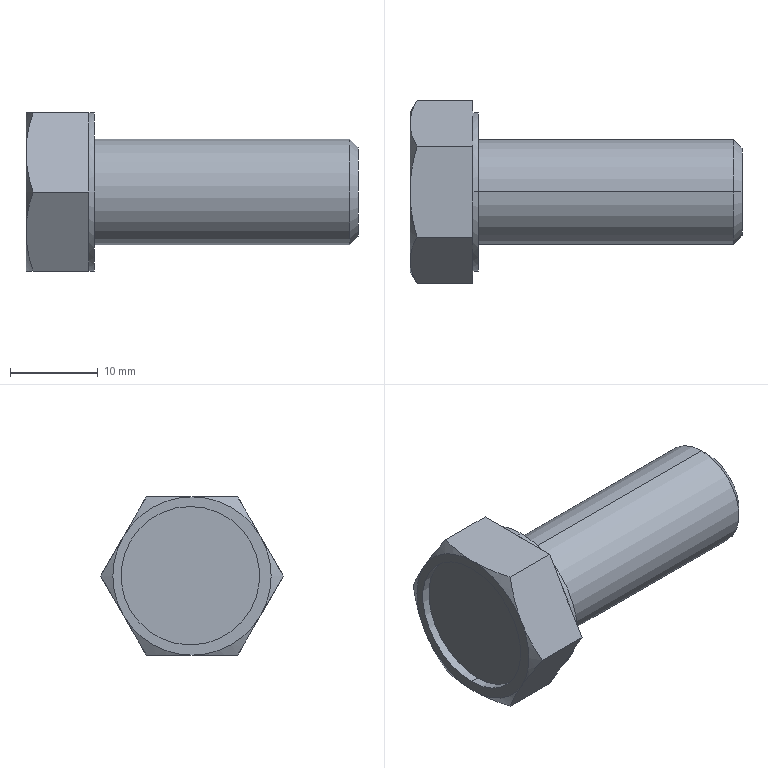Part | STEP file | formed hex screw_am_B18.2.3.2M - Formed hex screw, M12 x 1.75 x 30 --30WN | 1 solid | 30 faces | box 37.76 x 20.785 x 18 mm | volume 5343 mm3 | plane 16 | cone 8 | cylinder 6 | commonest cylinder face diameters 12 x2 15.75 x2 18 x2